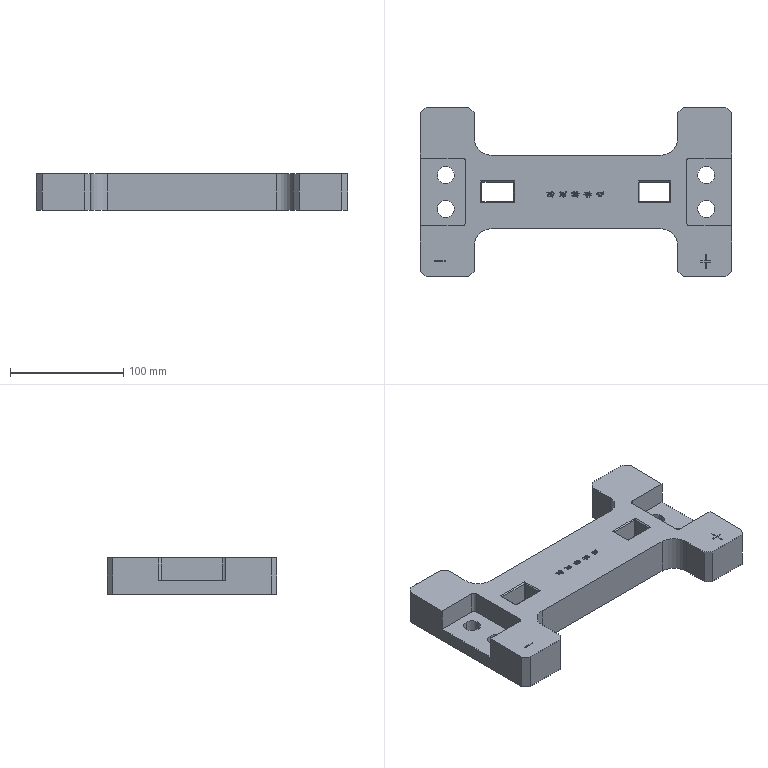CAM job | NX | 3-axis milling, drilling | part box 275 x 150 x 32 mm | stock box 275 x 150 x 32 mm
Tools:
number,name,description,diameter,corner_radius,flute_length,length,flutes
10,D10,Milling Tool-5 Parameters,10.0,0.0,50.0,75.0,2
21,D17R0.8,Milling Tool-5 Parameters,17.0,0.8,50.0,75.0,2
11,D10JING,Milling Tool-5 Parameters,10.0,0.0,50.0,75.0,2
6,D6,Milling Tool-5 Parameters,6.0,0.0,50.0,75.0,2
1,ZXZ,Milling Tool-5 Parameters,6.0,0.0,50.0,75.0,2
22,D6A45,Milling Tool-5 Parameters,6.0,0.0,3.0,3.0,2
Operations:
program,operation,operation_type,tool,method,geometry_group,spindle_rpm,surface_speed,feed_per_tooth,feed_cut,feed_plunge,cut_length_mm,path_length_mm,cut_time_min,machine_time_min
1,FLOOR_WALL,VolumeBased25DMillingOperation,D17R0.8,METHOD,A,2000.0,106.0,0.5,2000.0,1000.0,30459.118,33188.753,16.06,16.333
1,ZLEVEL_PROFILE,ZLevelMilling,D17R0.8,METHOD,A,2000.0,106.0,0.5,2000.0,100.0,65575.349,67300.77,32.788,32.96
1,DRILLING_COPY_1_COPY_1,Operation,ZXZ,METHOD,A,5000.0,94.0,0.025,250.0,0.0,24.0,465.758,0.096,0.1402
1,ZLEVEL_PROFILE_COPY,ZLevelMilling,D10,METHOD,A,3000.0,94.0,0.25,1500.0,100.0,4853.695,7178.465,3.236,3.468
1,ZLEVEL_PROFILE_COPY_COPY,ZLevelMilling,D6,METHOD,A,4000.0,75.0,0.175,1400.0,100.0,6376.028,9778.553,4.554,4.895
1,FLOOR_WALL_1_1_COPY,VolumeBased25DMillingOperation,D10JING,METHOD,A,7000.0,219.0,0.0714,1000.0,100.0,1237.807,2041.124,1.238,1.318
1,ZLEVEL_PROFILE_1_COPY_COPY,ZLevelMilling,D10JING,METHOD,A,7500.0,141.0,0.0833,1250.0,100.0,1154.513,3587.097,0.9236,1.167
1,ZLEVEL_PROFILE_1_COPY_1_COPY,ZLevelMilling,D6A45,METHOD,A,7500.0,141.0,0.0667,1000.0,100.0,1137.072,1197.072,1.137,1.143
1,ZLEVEL_PROFILE_1_COPY_1_COPY_COPY,ZLevelMilling,D6A45,METHOD,A,7500.0,141.0,0.0667,1000.0,100.0,117.908,596.51,0.1179,0.1658